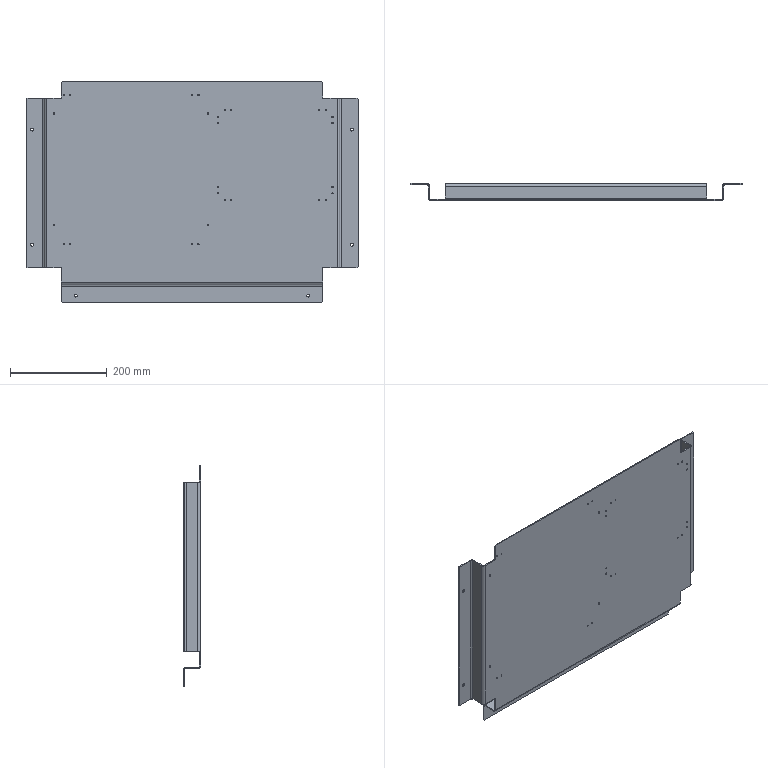Part | STEP file | 227H056121 BKT_Default | 1 solid | 138 faces | box 685.4 x 35.3 x 457.7 mm | volume 768690 mm3 | cylinder 80 | plane 58 | commonest cylinder face diameters 2.5 x48 6 x18 3.3 x8 10.6 x6